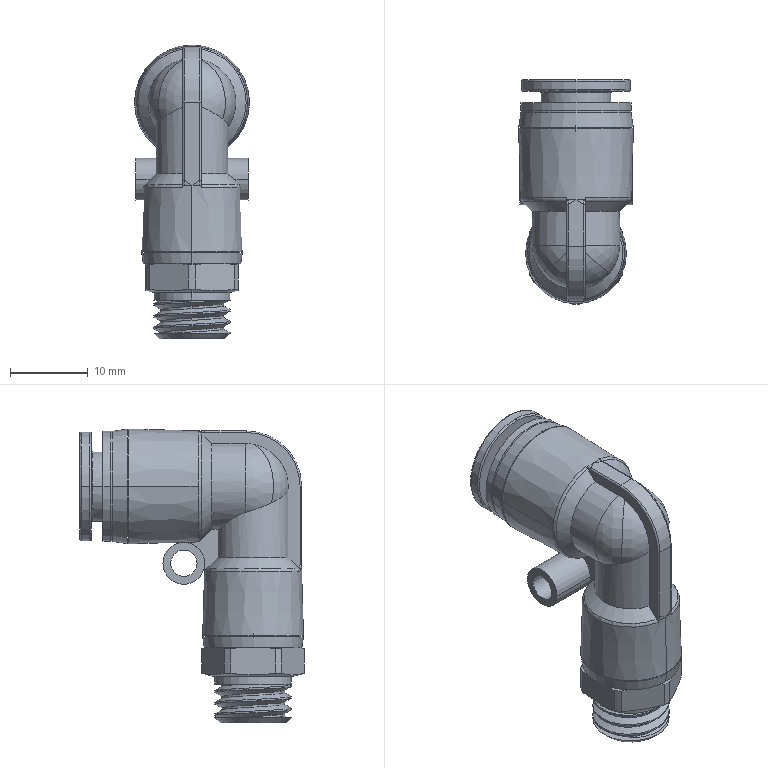Part | SolidWorks | features BaseBody 4 | 4 solids | 159 faces | box 14.797 x 28.95 x 37.899 mm | volume 4262 mm3 | cylinder 57 | plane 38 | cone 26 | torus 22 | spline 10 | sphere 6 | commonest cylinder face diameters 8 x7 8.141 x7 9.85 x7 13.2 x6 6.5 x5 14.2 x5